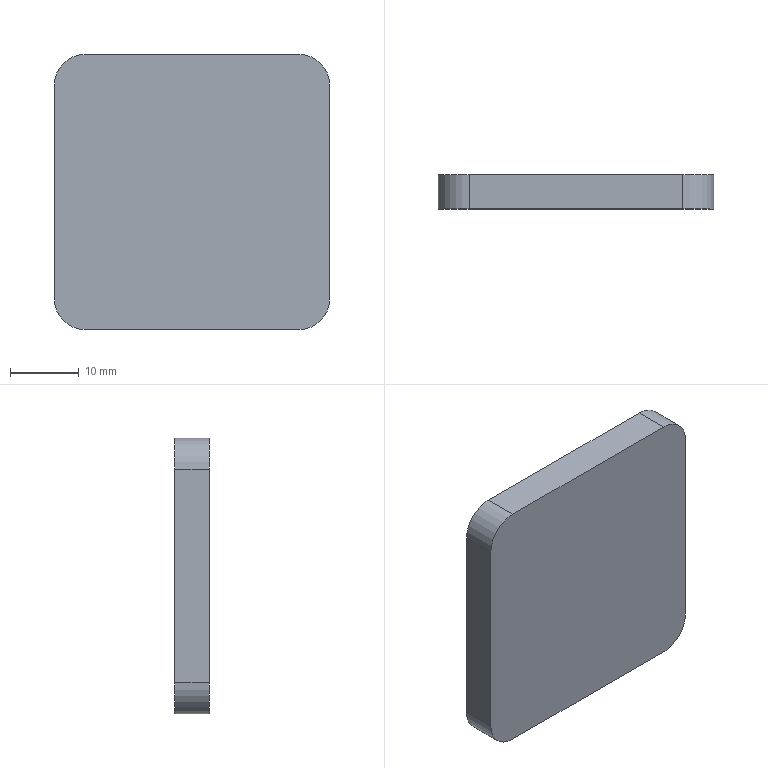Part | SolidWorks | features Extrusion 1, Fillet 1 | 1 solid | 10 faces | box 40 x 5 x 40 mm | volume 7913 mm3 | plane 6 | cylinder 4 | commonest cylinder face diameters 9 x4
STEP:
#1=CARTESIAN_POINT('',(20.,-2.5,15.5));
#2=VERTEX_POINT('',#1);
#3=CARTESIAN_POINT('',(20.,-2.5,-15.5));
#4=VERTEX_POINT('',#3);
#5=CARTESIAN_POINT('',(20.,-2.5,20.));
#6=DIRECTION('',(0.,0.,-1.));
#7=VECTOR('',#6,1000.);
#8=LINE('',#5,#7);
#9=EDGE_CURVE('',#2,#4,#8,.T.);
#10=ORIENTED_EDGE('',*,*,#9,.T.);
#11=CARTESIAN_POINT('',(20.,2.5,-15.5));
#12=VERTEX_POINT('',#11);
#13=CARTESIAN_POINT('',(20.,2.5,-15.5));
#14=DIRECTION('',(0.,1.,0.));
#15=VECTOR('',#14,1000.);
#16=LINE('',#13,#15);
#17=EDGE_CURVE('',#4,#12,#16,.T.);
#18=ORIENTED_EDGE('',*,*,#17,.T.);
#19=CARTESIAN_POINT('',(20.,2.5,15.5));
#20=VERTEX_POINT('',#19);
#21=CARTESIAN_POINT('',(20.,2.5,20.));
#22=DIRECTION('',(0.,0.,-1.));
#23=VECTOR('',#22,1000.);
#24=LINE('',#21,#23);
#25=EDGE_CURVE('',#20,#12,#24,.T.);
#26=ORIENTED_EDGE('',*,*,#25,.F.);
#27=CARTESIAN_POINT('',(20.,2.5,15.5));
#28=DIRECTION('',(0.,-1.,0.));
#29=VECTOR('',#28,1000.);
#30=LINE('',#27,#29);
#31=EDGE_CURVE('',#20,#2,#30,.T.);
#32=ORIENTED_EDGE('',*,*,#31,.T.);
#33=EDGE_LOOP('',(#10,#18,#26,#32));
#34=FACE_OUTER_BOUND('',#33,.T.);
#35=CARTESIAN_POINT('',(20.,2.5,20.));
#36=DIRECTION('',(-1.,0.,0.));
#37=DIRECTION('',(0.,0.,1.));
#38=AXIS2_PLACEMENT_3D('',#35,#36,#37);
#39=PLANE('',#38);
#40=ADVANCED_FACE('',(#34),#39,.F.);
#41=CARTESIAN_POINT('',(15.5,2.5,-20.));
#42=VERTEX_POINT('',#41);
#43=CARTESIAN_POINT('',(-15.5,2.5,-20.));
#44=VERTEX_POINT('',#43);
#45=CARTESIAN_POINT('',(-20.,2.5,-20.));
#46=DIRECTION('',(-1.,0.,0.));
#47=VECTOR('',#46,1000.);
#48=LINE('',#45,#47);
#49=EDGE_CURVE('',#42,#44,#48,.T.);
#50=ORIENTED_EDGE('',*,*,#49,.F.);
#51=CARTESIAN_POINT('',(15.5,-2.5,-20.));
#52=VERTEX_POINT('',#51);
#53=CARTESIAN_POINT('',(15.5,2.5,-20.));
#54=DIRECTION('',(0.,-1.,0.));
#55=VECTOR('',#54,1000.);
#56=LINE('',#53,#55);
#57=EDGE_CURVE('',#42,#52,#56,.T.);
#58=ORIENTED_EDGE('',*,*,#57,.T.);
#59=CARTESIAN_POINT('',(-15.5,-2.5,-20.));
#60=VERTEX_POINT('',#59);
#61=CARTESIAN_POINT('',(-20.,-2.5,-20.));
#62=DIRECTION('',(-1.,0.,0.));
#63=VECTOR('',#62,1000.);
#64=LINE('',#61,#63);
#65=EDGE_CURVE('',#52,#60,#64,.T.);
#66=ORIENTED_EDGE('',*,*,#65,.T.);
#67=CARTESIAN_POINT('',(-15.5,2.5,-20.));
#68=DIRECTION('',(0.,1.,0.));
#69=VECTOR('',#68,1000.);
#70=LINE('',#67,#69);
#71=EDGE_CURVE('',#60,#44,#70,.T.);
#72=ORIENTED_EDGE('',*,*,#71,.T.);
#73=EDGE_LOOP('',(#50,#58,#66,#72));
#74=FACE_OUTER_BOUND('',#73,.T.);
#75=CARTESIAN_POINT('',(-20.,2.5,-20.));
#76=DIRECTION('',(0.,0.,1.));
#77=DIRECTION('',(1.,0.,0.));
#78=AXIS2_PLACEMENT_3D('',#75,#76,#77);
#79=PLANE('',#78);
#80=ADVANCED_FACE('',(#74),#79,.F.);
#81=CARTESIAN_POINT('',(-20.,2.5,-15.5));
#82=VERTEX_POINT('',#81);
#83=CARTESIAN_POINT('',(-20.,2.5,15.5));
#84=VERTEX_POINT('',#83);
#85=CARTESIAN_POINT('',(-20.,2.5,20.));
#86=DIRECTION('',(0.,0.,1.));
#87=VECTOR('',#86,1000.);
#88=LINE('',#85,#87);
#89=EDGE_CURVE('',#82,#84,#88,.T.);
#90=ORIENTED_EDGE('',*,*,#89,.F.);
#91=CARTESIAN_POINT('',(-20.,-2.5,-15.5));
#92=VERTEX_POINT('',#91);
#93=CARTESIAN_POINT('',(-20.,2.5,-15.5));
#94=DIRECTION('',(0.,-1.,0.));
#95=VECTOR('',#94,1000.);
#96=LINE('',#93,#95);
#97=EDGE_CURVE('',#82,#92,#96,.T.);
#98=ORIENTED_EDGE('',*,*,#97,.T.);
#99=CARTESIAN_POINT('',(-20.,-2.5,15.5));
#100=VERTEX_POINT('',#99);
#101=CARTESIAN_POINT('',(-20.,-2.5,20.));
#102=DIRECTION('',(0.,0.,1.));
#103=VECTOR('',#102,1000.);
#104=LINE('',#101,#103);
#105=EDGE_CURVE('',#92,#100,#104,.T.);
#106=ORIENTED_EDGE('',*,*,#105,.T.);
#107=CARTESIAN_POINT('',(-20.,2.5,15.5));
#108=DIRECTION('',(0.,1.,0.));
#109=VECTOR('',#108,1000.);
#110=LINE('',#107,#109);
#111=EDGE_CURVE('',#100,#84,#110,.T.);
#112=ORIENTED_EDGE('',*,*,#111,.T.);
#113=EDGE_LOOP('',(#90,#98,#106,#112));
#114=FACE_OUTER_BOUND('',#113,.T.);
#115=CARTESIAN_POINT('',(-20.,2.5,20.));
#116=DIRECTION('',(1.,0.,0.));
#117=DIRECTION('',(0.,0.,-1.));
#118=AXIS2_PLACEMENT_3D('',#115,#116,#117);
#119=PLANE('',#118);
#120=ADVANCED_FACE('',(#114),#119,.F.);
#121=CARTESIAN_POINT('',(-15.5,-2.5,20.));
#122=VERTEX_POINT('',#121);
#123=CARTESIAN_POINT('',(15.5,-2.5,20.));
#124=VERTEX_POINT('',#123);
#125=CARTESIAN_POINT('',(-20.,-2.5,20.));
#126=DIRECTION('',(1.,0.,0.));
#127=VECTOR('',#126,1000.);
#128=LINE('',#125,#127);
#129=EDGE_CURVE('',#122,#124,#128,.T.);
#130=ORIENTED_EDGE('',*,*,#129,.T.);
#131=CARTESIAN_POINT('',(15.5,2.5,20.));
#132=VERTEX_POINT('',#131);
#133=CARTESIAN_POINT('',(15.5,2.5,20.));
#134=DIRECTION('',(0.,1.,0.));
#135=VECTOR('',#134,1000.);
#136=LINE('',#133,#135);
#137=EDGE_CURVE('',#124,#132,#136,.T.);
#138=ORIENTED_EDGE('',*,*,#137,.T.);
#139=CARTESIAN_POINT('',(-15.5,2.5,20.));
#140=VERTEX_POINT('',#139);
#141=CARTESIAN_POINT('',(-20.,2.5,20.));
#142=DIRECTION('',(1.,0.,0.));
#143=VECTOR('',#142,1000.);
#144=LINE('',#141,#143);
#145=EDGE_CURVE('',#140,#132,#144,.T.);
#146=ORIENTED_EDGE('',*,*,#145,.F.);
#147=CARTESIAN_POINT('',(-15.5,2.5,20.));
#148=DIRECTION('',(0.,-1.,0.));
#149=VECTOR('',#148,1000.);
#150=LINE('',#147,#149);
#151=EDGE_CURVE('',#140,#122,#150,.T.);
#152=ORIENTED_EDGE('',*,*,#151,.T.);
#153=EDGE_LOOP('',(#130,#138,#146,#152));
#154=FACE_OUTER_BOUND('',#153,.T.);
#155=CARTESIAN_POINT('',(-20.,2.5,20.));
#156=DIRECTION('',(0.,0.,-1.));
#157=DIRECTION('',(-1.,0.,0.));
#158=AXIS2_PLACEMENT_3D('',#155,#156,#157);
#159=PLANE('',#158);
#160=ADVANCED_FACE('',(#154),#159,.F.);
#161=ORIENTED_EDGE('',*,*,#25,.T.);
#162=CARTESIAN_POINT('',(15.5,2.5,-15.5));
#163=DIRECTION('',(0.,1.,0.));
#164=DIRECTION('',(0.,0.,-1.));
#165=AXIS2_PLACEMENT_3D('',#162,#163,#164);
#166=CIRCLE('',#165,4.5);
#167=EDGE_CURVE('',#12,#42,#166,.T.);
#168=ORIENTED_EDGE('',*,*,#167,.T.);
#169=ORIENTED_EDGE('',*,*,#49,.T.);
#170=CARTESIAN_POINT('',(-15.5,2.5,-15.5));
#171=DIRECTION('',(0.,1.,0.));
#172=DIRECTION('',(0.,0.,-1.));
#173=AXIS2_PLACEMENT_3D('',#170,#171,#172);
#174=CIRCLE('',#173,4.5);
#175=EDGE_CURVE('',#44,#82,#174,.T.);
#176=ORIENTED_EDGE('',*,*,#175,.T.);
#177=ORIENTED_EDGE('',*,*,#89,.T.);
#178=CARTESIAN_POINT('',(-15.5,2.5,15.5));
#179=DIRECTION('',(0.,1.,0.));
#180=DIRECTION('',(0.,0.,-1.));
#181=AXIS2_PLACEMENT_3D('',#178,#179,#180);
#182=CIRCLE('',#181,4.5);
#183=EDGE_CURVE('',#84,#140,#182,.T.);
#184=ORIENTED_EDGE('',*,*,#183,.T.);
#185=ORIENTED_EDGE('',*,*,#145,.T.);
#186=CARTESIAN_POINT('',(15.5,2.5,15.5));
#187=DIRECTION('',(0.,1.,0.));
#188=DIRECTION('',(0.,0.,-1.));
#189=AXIS2_PLACEMENT_3D('',#186,#187,#188);
#190=CIRCLE('',#189,4.5);
#191=EDGE_CURVE('',#132,#20,#190,.T.);
#192=ORIENTED_EDGE('',*,*,#191,.T.);
#193=EDGE_LOOP('',(#161,#168,#169,#176,#177,#184,#185,#192));
#194=FACE_OUTER_BOUND('',#193,.T.);
#195=CARTESIAN_POINT('',(0.,2.5,0.));
#196=DIRECTION('',(0.,-1.,0.));
#197=DIRECTION('',(0.,0.,-1.));
#198=AXIS2_PLACEMENT_3D('',#195,#196,#197);
#199=PLANE('',#198);
#200=ADVANCED_FACE('',(#194),#199,.F.);
#201=ORIENTED_EDGE('',*,*,#65,.F.);
#202=CARTESIAN_POINT('',(15.5,-2.5,-15.5));
#203=DIRECTION('',(0.,-1.,0.));
#204=DIRECTION('',(0.,0.,-1.));
#205=AXIS2_PLACEMENT_3D('',#202,#203,#204);
#206=CIRCLE('',#205,4.5);
#207=EDGE_CURVE('',#52,#4,#206,.T.);
#208=ORIENTED_EDGE('',*,*,#207,.T.);
#209=ORIENTED_EDGE('',*,*,#9,.F.);
#210=CARTESIAN_POINT('',(15.5,-2.5,15.5));
#211=DIRECTION('',(0.,-1.,0.));
#212=DIRECTION('',(0.,0.,-1.));
#213=AXIS2_PLACEMENT_3D('',#210,#211,#212);
#214=CIRCLE('',#213,4.5);
#215=EDGE_CURVE('',#2,#124,#214,.T.);
#216=ORIENTED_EDGE('',*,*,#215,.T.);
#217=ORIENTED_EDGE('',*,*,#129,.F.);
#218=CARTESIAN_POINT('',(-15.5,-2.5,15.5));
#219=DIRECTION('',(0.,-1.,0.));
#220=DIRECTION('',(0.,0.,-1.));
#221=AXIS2_PLACEMENT_3D('',#218,#219,#220);
#222=CIRCLE('',#221,4.5);
#223=EDGE_CURVE('',#122,#100,#222,.T.);
#224=ORIENTED_EDGE('',*,*,#223,.T.);
#225=ORIENTED_EDGE('',*,*,#105,.F.);
#226=CARTESIAN_POINT('',(-15.5,-2.5,-15.5));
#227=DIRECTION('',(0.,-1.,0.));
#228=DIRECTION('',(0.,0.,-1.));
#229=AXIS2_PLACEMENT_3D('',#226,#227,#228);
#230=CIRCLE('',#229,4.5);
#231=EDGE_CURVE('',#92,#60,#230,.T.);
#232=ORIENTED_EDGE('',*,*,#231,.T.);
#233=EDGE_LOOP('',(#201,#208,#209,#216,#217,#224,#225,#232));
#234=FACE_OUTER_BOUND('',#233,.T.);
#235=CARTESIAN_POINT('',(0.,-2.5,0.));
#236=DIRECTION('',(0.,-1.,0.));
#237=DIRECTION('',(0.,0.,-1.));
#238=AXIS2_PLACEMENT_3D('',#235,#236,#237);
#239=PLANE('',#238);
#240=ADVANCED_FACE('',(#234),#239,.T.);
#241=ORIENTED_EDGE('',*,*,#167,.F.);
#242=ORIENTED_EDGE('',*,*,#17,.F.);
#243=ORIENTED_EDGE('',*,*,#207,.F.);
#244=ORIENTED_EDGE('',*,*,#57,.F.);
#245=EDGE_LOOP('',(#241,#242,#243,#244));
#246=FACE_OUTER_BOUND('',#245,.T.);
#247=CARTESIAN_POINT('',(15.5,2.5,-15.5));
#248=DIRECTION('',(0.,-1.,0.));
#249=DIRECTION('',(0.,0.,-1.));
#250=AXIS2_PLACEMENT_3D('',#247,#248,#249);
#251=CYLINDRICAL_SURFACE('',#250,4.5);
#252=ADVANCED_FACE('',(#246),#251,.T.);
#253=ORIENTED_EDGE('',*,*,#191,.F.);
#254=ORIENTED_EDGE('',*,*,#137,.F.);
#255=ORIENTED_EDGE('',*,*,#215,.F.);
#256=ORIENTED_EDGE('',*,*,#31,.F.);
#257=EDGE_LOOP('',(#253,#254,#255,#256));
#258=FACE_OUTER_BOUND('',#257,.T.);
#259=CARTESIAN_POINT('',(15.5,2.5,15.5));
#260=DIRECTION('',(0.,-1.,0.));
#261=DIRECTION('',(0.,0.,-1.));
#262=AXIS2_PLACEMENT_3D('',#259,#260,#261);
#263=CYLINDRICAL_SURFACE('',#262,4.5);
#264=ADVANCED_FACE('',(#258),#263,.T.);
#265=ORIENTED_EDGE('',*,*,#175,.F.);
#266=ORIENTED_EDGE('',*,*,#71,.F.);
#267=ORIENTED_EDGE('',*,*,#231,.F.);
#268=ORIENTED_EDGE('',*,*,#97,.F.);
#269=EDGE_LOOP('',(#265,#266,#267,#268));
#270=FACE_OUTER_BOUND('',#269,.T.);
#271=CARTESIAN_POINT('',(-15.5,2.5,-15.5));
#272=DIRECTION('',(0.,-1.,0.));
#273=DIRECTION('',(0.,0.,-1.));
#274=AXIS2_PLACEMENT_3D('',#271,#272,#273);
#275=CYLINDRICAL_SURFACE('',#274,4.5);
#276=ADVANCED_FACE('',(#270),#275,.T.);
#277=ORIENTED_EDGE('',*,*,#183,.F.);
#278=ORIENTED_EDGE('',*,*,#111,.F.);
#279=ORIENTED_EDGE('',*,*,#223,.F.);
#280=ORIENTED_EDGE('',*,*,#151,.F.);
#281=EDGE_LOOP('',(#277,#278,#279,#280));
#282=FACE_OUTER_BOUND('',#281,.T.);
#283=CARTESIAN_POINT('',(-15.5,2.5,15.5));
#284=DIRECTION('',(0.,-1.,0.));
#285=DIRECTION('',(0.,0.,-1.));
#286=AXIS2_PLACEMENT_3D('',#283,#284,#285);
#287=CYLINDRICAL_SURFACE('',#286,4.5);
#288=ADVANCED_FACE('',(#282),#287,.T.);
#289=CLOSED_SHELL('',(#40,#80,#120,#160,#200,#240,#252,#264,#276,#288));
#290=MANIFOLD_SOLID_BREP('',#289);
#291=CARTESIAN_POINT('',(0.,0.,0.));
#292=DIRECTION('',(0.,0.,1.));
#293=DIRECTION('',(1.,0.,0.));
#294=AXIS2_PLACEMENT_3D('',#291,#292,#293);
#295=(LENGTH_UNIT()NAMED_UNIT(*)SI_UNIT(.MILLI.,.METRE.));
#296=UNCERTAINTY_MEASURE_WITH_UNIT(LENGTH_MEASURE(0.00001),#295,'','');
#297=(NAMED_UNIT(*)PLANE_ANGLE_UNIT()SI_UNIT($,.RADIAN.));
#298=(NAMED_UNIT(*)SI_UNIT($,.STERADIAN.)SOLID_ANGLE_UNIT());
#299=(GEOMETRIC_REPRESENTATION_CONTEXT(3)GLOBAL_UNCERTAINTY_ASSIGNED_CONTEXT((#296))GLOBAL_UNIT_ASSIGNED_CONTEXT((#295,#297,#298))REPRESENTATION_CONTEXT('',''));
#300=ADVANCED_BREP_SHAPE_REPRESENTATION('',(#290,#294),#299);